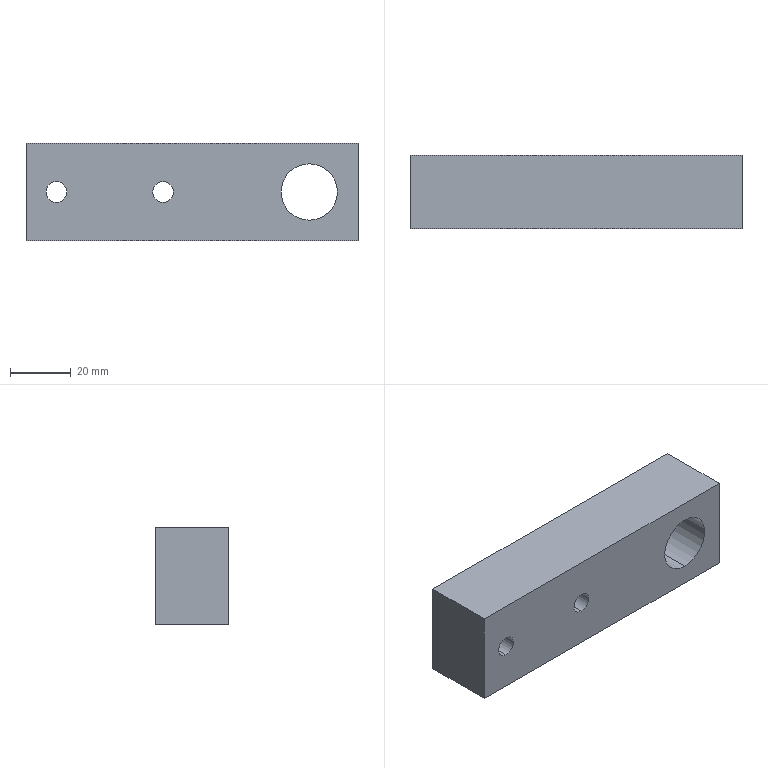Part | STEP file | PN_0035 (buffer fixed block) | 1 solid | 12 faces | box 109 x 24 x 32 mm | volume 75518 mm3 | cylinder 6 | plane 6 | commonest cylinder face diameters 6.8 x4 18.5 x2
STEP:
#1=CARTESIAN_POINT('',(0.,0.,0.));
#2=DIRECTION('',(0.,0.,1.));
#3=DIRECTION('',(1.,0.,0.));
#4=AXIS2_PLACEMENT_3D('',#1,#2,#3);
#5=CARTESIAN_POINT('',(10.,-12.,3.4));
#6=VERTEX_POINT('',#5);
#7=CARTESIAN_POINT('',(10.,12.,3.4));
#8=VERTEX_POINT('',#7);
#9=CARTESIAN_POINT('',(10.,12.,3.4));
#10=DIRECTION('',(0.,1.,0.));
#11=VECTOR('',#10,1.);
#12=LINE('',#9,#11);
#13=CARTESIAN_POINT('',(10.,12.,0.));
#14=DIRECTION('',(0.,1.,0.));
#15=DIRECTION('',(0.,0.,1.));
#16=AXIS2_PLACEMENT_3D('',#13,#14,#15);
#17=CYLINDRICAL_SURFACE('',#16,3.4);
#18=CARTESIAN_POINT('',(6.283,0.));
#19=DIRECTION('',(0.,1.));
#20=VECTOR('',#19,1.);
#21=LINE('',#18,#20);
#22=(GEOMETRIC_REPRESENTATION_CONTEXT(2)PARAMETRIC_REPRESENTATION_CONTEXT()REPRESENTATION_CONTEXT('',''));
#23=DEFINITIONAL_REPRESENTATION('',(#21),#22);
#24=PCURVE('',#17,#23);
#25=CARTESIAN_POINT('',(10.,12.,0.));
#26=DIRECTION('',(0.,1.,0.));
#27=DIRECTION('',(0.,0.,1.));
#28=AXIS2_PLACEMENT_3D('',#25,#26,#27);
#29=CYLINDRICAL_SURFACE('',#28,3.4);
#30=CARTESIAN_POINT('',(0.,0.));
#31=DIRECTION('',(0.,1.));
#32=VECTOR('',#31,1.);
#33=LINE('',#30,#32);
#34=(GEOMETRIC_REPRESENTATION_CONTEXT(2)PARAMETRIC_REPRESENTATION_CONTEXT()REPRESENTATION_CONTEXT('',''));
#35=DEFINITIONAL_REPRESENTATION('',(#33),#34);
#36=PCURVE('',#29,#35);
#37=SURFACE_CURVE('',#12,(#24,#36),.PCURVE_S1.);
#38=EDGE_CURVE('',#6,#8,#37,.T.);
#39=ORIENTED_EDGE('',*,*,#38,.T.);
#40=CARTESIAN_POINT('',(10.,12.,-3.4));
#41=VERTEX_POINT('',#40);
#42=CARTESIAN_POINT('',(10.,12.,0.));
#43=DIRECTION('',(0.,1.,0.));
#44=DIRECTION('',(0.,0.,1.));
#45=AXIS2_PLACEMENT_3D('',#42,#43,#44);
#46=CIRCLE('',#45,3.4);
#47=CARTESIAN_POINT('',(0.,0.));
#48=DIRECTION('',(1.,0.));
#49=VECTOR('',#48,1.);
#50=LINE('',#47,#49);
#51=(GEOMETRIC_REPRESENTATION_CONTEXT(2)PARAMETRIC_REPRESENTATION_CONTEXT()REPRESENTATION_CONTEXT('',''));
#52=DEFINITIONAL_REPRESENTATION('',(#50),#51);
#53=PCURVE('',#17,#52);
#54=CARTESIAN_POINT('',(0.,12.,16.));
#55=DIRECTION('',(0.,-1.,0.));
#56=DIRECTION('',(0.,0.,-1.));
#57=AXIS2_PLACEMENT_3D('',#54,#55,#56);
#58=PLANE('',#57);
#59=CARTESIAN_POINT('',(12.6,10.));
#60=CARTESIAN_POINT('',(12.6,15.889));
#61=CARTESIAN_POINT('',(17.7,12.944));
#62=CARTESIAN_POINT('',(22.8,10.));
#63=CARTESIAN_POINT('',(17.7,7.056));
#64=CARTESIAN_POINT('',(12.6,4.111));
#65=CARTESIAN_POINT('',(12.6,10.));
#66=(BOUNDED_CURVE()B_SPLINE_CURVE(2,(#59,#60,#61,#62,#63,#64,#65),.UNSPECIFIED.,.T.,.F.)B_SPLINE_CURVE_WITH_KNOTS((1,2,2,2,2,1),(-2.094,0.,2.094,4.189,6.283,8.378),.UNSPECIFIED.)CURVE()GEOMETRIC_REPRESENTATION_ITEM()RATIONAL_B_SPLINE_CURVE((1.,0.5,1.,0.5,1.,0.5,1.))REPRESENTATION_ITEM(''));
#67=(GEOMETRIC_REPRESENTATION_CONTEXT(2)PARAMETRIC_REPRESENTATION_CONTEXT()REPRESENTATION_CONTEXT('',''));
#68=DEFINITIONAL_REPRESENTATION('',(#66),#67);
#69=PCURVE('',#58,#68);
#70=SURFACE_CURVE('',#46,(#53,#69),.PCURVE_S1.);
#71=EDGE_CURVE('',#41,#8,#70,.T.);
#72=ORIENTED_EDGE('',*,*,#71,.F.);
#73=CARTESIAN_POINT('',(10.,-12.,-3.4));
#74=VERTEX_POINT('',#73);
#75=CARTESIAN_POINT('',(10.,12.,-3.4));
#76=DIRECTION('',(0.,1.,0.));
#77=VECTOR('',#76,1.);
#78=LINE('',#75,#77);
#79=CARTESIAN_POINT('',(3.142,0.));
#80=DIRECTION('',(0.,1.));
#81=VECTOR('',#80,1.);
#82=LINE('',#79,#81);
#83=(GEOMETRIC_REPRESENTATION_CONTEXT(2)PARAMETRIC_REPRESENTATION_CONTEXT()REPRESENTATION_CONTEXT('',''));
#84=DEFINITIONAL_REPRESENTATION('',(#82),#83);
#85=PCURVE('',#17,#84);
#86=CARTESIAN_POINT('',(3.142,0.));
#87=DIRECTION('',(0.,1.));
#88=VECTOR('',#87,1.);
#89=LINE('',#86,#88);
#90=(GEOMETRIC_REPRESENTATION_CONTEXT(2)PARAMETRIC_REPRESENTATION_CONTEXT()REPRESENTATION_CONTEXT('',''));
#91=DEFINITIONAL_REPRESENTATION('',(#89),#90);
#92=PCURVE('',#29,#91);
#93=SURFACE_CURVE('',#78,(#85,#92),.PCURVE_S1.);
#94=EDGE_CURVE('',#74,#41,#93,.T.);
#95=ORIENTED_EDGE('',*,*,#94,.F.);
#96=CARTESIAN_POINT('',(10.,-12.,0.));
#97=DIRECTION('',(0.,1.,0.));
#98=DIRECTION('',(0.,0.,1.));
#99=AXIS2_PLACEMENT_3D('',#96,#97,#98);
#100=CIRCLE('',#99,3.4);
#101=CARTESIAN_POINT('',(0.,-24.));
#102=DIRECTION('',(1.,0.));
#103=VECTOR('',#102,1.);
#104=LINE('',#101,#103);
#105=(GEOMETRIC_REPRESENTATION_CONTEXT(2)PARAMETRIC_REPRESENTATION_CONTEXT()REPRESENTATION_CONTEXT('',''));
#106=DEFINITIONAL_REPRESENTATION('',(#104),#105);
#107=PCURVE('',#17,#106);
#108=CARTESIAN_POINT('',(0.,-12.,16.));
#109=DIRECTION('',(0.,1.,0.));
#110=DIRECTION('',(0.,0.,1.));
#111=AXIS2_PLACEMENT_3D('',#108,#109,#110);
#112=PLANE('',#111);
#113=CARTESIAN_POINT('',(-16.,10.));
#114=DIRECTION('',(1.,0.));
#115=AXIS2_PLACEMENT_2D('',#113,#114);
#116=CIRCLE('',#115,3.4);
#117=(GEOMETRIC_REPRESENTATION_CONTEXT(2)PARAMETRIC_REPRESENTATION_CONTEXT()REPRESENTATION_CONTEXT('',''));
#118=DEFINITIONAL_REPRESENTATION('',(#116),#117);
#119=PCURVE('',#112,#118);
#120=SURFACE_CURVE('',#100,(#107,#119),.PCURVE_S1.);
#121=EDGE_CURVE('',#74,#6,#120,.T.);
#122=ORIENTED_EDGE('',*,*,#121,.T.);
#123=EDGE_LOOP('',(#39,#72,#95,#122));
#124=FACE_BOUND('',#123,.F.);
#125=ADVANCED_FACE('',(#124),#17,.F.);
#126=CARTESIAN_POINT('',(45.,-12.,3.4));
#127=VERTEX_POINT('',#126);
#128=CARTESIAN_POINT('',(45.,12.,3.4));
#129=VERTEX_POINT('',#128);
#130=CARTESIAN_POINT('',(45.,12.,3.4));
#131=DIRECTION('',(0.,1.,0.));
#132=VECTOR('',#131,1.);
#133=LINE('',#130,#132);
#134=CARTESIAN_POINT('',(45.,12.,0.));
#135=DIRECTION('',(0.,1.,0.));
#136=DIRECTION('',(0.,0.,1.));
#137=AXIS2_PLACEMENT_3D('',#134,#135,#136);
#138=CYLINDRICAL_SURFACE('',#137,3.4);
#139=CARTESIAN_POINT('',(6.283,0.));
#140=DIRECTION('',(0.,1.));
#141=VECTOR('',#140,1.);
#142=LINE('',#139,#141);
#143=(GEOMETRIC_REPRESENTATION_CONTEXT(2)PARAMETRIC_REPRESENTATION_CONTEXT()REPRESENTATION_CONTEXT('',''));
#144=DEFINITIONAL_REPRESENTATION('',(#142),#143);
#145=PCURVE('',#138,#144);
#146=CARTESIAN_POINT('',(45.,12.,0.));
#147=DIRECTION('',(0.,1.,0.));
#148=DIRECTION('',(0.,0.,1.));
#149=AXIS2_PLACEMENT_3D('',#146,#147,#148);
#150=CYLINDRICAL_SURFACE('',#149,3.4);
#151=CARTESIAN_POINT('',(0.,0.));
#152=DIRECTION('',(0.,1.));
#153=VECTOR('',#152,1.);
#154=LINE('',#151,#153);
#155=(GEOMETRIC_REPRESENTATION_CONTEXT(2)PARAMETRIC_REPRESENTATION_CONTEXT()REPRESENTATION_CONTEXT('',''));
#156=DEFINITIONAL_REPRESENTATION('',(#154),#155);
#157=PCURVE('',#150,#156);
#158=SURFACE_CURVE('',#133,(#145,#157),.PCURVE_S1.);
#159=EDGE_CURVE('',#127,#129,#158,.T.);
#160=ORIENTED_EDGE('',*,*,#159,.T.);
#161=CARTESIAN_POINT('',(45.,12.,-3.4));
#162=VERTEX_POINT('',#161);
#163=CARTESIAN_POINT('',(45.,12.,0.));
#164=DIRECTION('',(0.,1.,0.));
#165=DIRECTION('',(0.,0.,1.));
#166=AXIS2_PLACEMENT_3D('',#163,#164,#165);
#167=CIRCLE('',#166,3.4);
#168=CARTESIAN_POINT('',(0.,0.));
#169=DIRECTION('',(1.,0.));
#170=VECTOR('',#169,1.);
#171=LINE('',#168,#170);
#172=(GEOMETRIC_REPRESENTATION_CONTEXT(2)PARAMETRIC_REPRESENTATION_CONTEXT()REPRESENTATION_CONTEXT('',''));
#173=DEFINITIONAL_REPRESENTATION('',(#171),#172);
#174=PCURVE('',#138,#173);
#175=CARTESIAN_POINT('',(12.6,45.));
#176=CARTESIAN_POINT('',(12.6,50.889));
#177=CARTESIAN_POINT('',(17.7,47.944));
#178=CARTESIAN_POINT('',(22.8,45.));
#179=CARTESIAN_POINT('',(17.7,42.056));
#180=CARTESIAN_POINT('',(12.6,39.111));
#181=CARTESIAN_POINT('',(12.6,45.));
#182=(BOUNDED_CURVE()B_SPLINE_CURVE(2,(#175,#176,#177,#178,#179,#180,#181),.UNSPECIFIED.,.T.,.F.)B_SPLINE_CURVE_WITH_KNOTS((1,2,2,2,2,1),(-2.094,0.,2.094,4.189,6.283,8.378),.UNSPECIFIED.)CURVE()GEOMETRIC_REPRESENTATION_ITEM()RATIONAL_B_SPLINE_CURVE((1.,0.5,1.,0.5,1.,0.5,1.))REPRESENTATION_ITEM(''));
#183=(GEOMETRIC_REPRESENTATION_CONTEXT(2)PARAMETRIC_REPRESENTATION_CONTEXT()REPRESENTATION_CONTEXT('',''));
#184=DEFINITIONAL_REPRESENTATION('',(#182),#183);
#185=PCURVE('',#58,#184);
#186=SURFACE_CURVE('',#167,(#174,#185),.PCURVE_S1.);
#187=EDGE_CURVE('',#162,#129,#186,.T.);
#188=ORIENTED_EDGE('',*,*,#187,.F.);
#189=CARTESIAN_POINT('',(45.,-12.,-3.4));
#190=VERTEX_POINT('',#189);
#191=CARTESIAN_POINT('',(45.,12.,-3.4));
#192=DIRECTION('',(0.,1.,0.));
#193=VECTOR('',#192,1.);
#194=LINE('',#191,#193);
#195=CARTESIAN_POINT('',(3.142,0.));
#196=DIRECTION('',(0.,1.));
#197=VECTOR('',#196,1.);
#198=LINE('',#195,#197);
#199=(GEOMETRIC_REPRESENTATION_CONTEXT(2)PARAMETRIC_REPRESENTATION_CONTEXT()REPRESENTATION_CONTEXT('',''));
#200=DEFINITIONAL_REPRESENTATION('',(#198),#199);
#201=PCURVE('',#138,#200);
#202=CARTESIAN_POINT('',(3.142,0.));
#203=DIRECTION('',(0.,1.));
#204=VECTOR('',#203,1.);
#205=LINE('',#202,#204);
#206=(GEOMETRIC_REPRESENTATION_CONTEXT(2)PARAMETRIC_REPRESENTATION_CONTEXT()REPRESENTATION_CONTEXT('',''));
#207=DEFINITIONAL_REPRESENTATION('',(#205),#206);
#208=PCURVE('',#150,#207);
#209=SURFACE_CURVE('',#194,(#201,#208),.PCURVE_S1.);
#210=EDGE_CURVE('',#190,#162,#209,.T.);
#211=ORIENTED_EDGE('',*,*,#210,.F.);
#212=CARTESIAN_POINT('',(45.,-12.,0.));
#213=DIRECTION('',(0.,1.,0.));
#214=DIRECTION('',(0.,0.,1.));
#215=AXIS2_PLACEMENT_3D('',#212,#213,#214);
#216=CIRCLE('',#215,3.4);
#217=CARTESIAN_POINT('',(0.,-24.));
#218=DIRECTION('',(1.,0.));
#219=VECTOR('',#218,1.);
#220=LINE('',#217,#219);
#221=(GEOMETRIC_REPRESENTATION_CONTEXT(2)PARAMETRIC_REPRESENTATION_CONTEXT()REPRESENTATION_CONTEXT('',''));
#222=DEFINITIONAL_REPRESENTATION('',(#220),#221);
#223=PCURVE('',#138,#222);
#224=CARTESIAN_POINT('',(-16.,45.));
#225=DIRECTION('',(1.,0.));
#226=AXIS2_PLACEMENT_2D('',#224,#225);
#227=CIRCLE('',#226,3.4);
#228=(GEOMETRIC_REPRESENTATION_CONTEXT(2)PARAMETRIC_REPRESENTATION_CONTEXT()REPRESENTATION_CONTEXT('',''));
#229=DEFINITIONAL_REPRESENTATION('',(#227),#228);
#230=PCURVE('',#112,#229);
#231=SURFACE_CURVE('',#216,(#223,#230),.PCURVE_S1.);
#232=EDGE_CURVE('',#190,#127,#231,.T.);
#233=ORIENTED_EDGE('',*,*,#232,.T.);
#234=EDGE_LOOP('',(#160,#188,#211,#233));
#235=FACE_BOUND('',#234,.F.);
#236=ADVANCED_FACE('',(#235),#138,.F.);
#237=CARTESIAN_POINT('',(93.,-12.,9.25));
#238=VERTEX_POINT('',#237);
#239=CARTESIAN_POINT('',(93.,12.,9.25));
#240=VERTEX_POINT('',#239);
#241=CARTESIAN_POINT('',(93.,12.,9.25));
#242=DIRECTION('',(0.,1.,0.));
#243=VECTOR('',#242,1.);
#244=LINE('',#241,#243);
#245=CARTESIAN_POINT('',(93.,12.,0.));
#246=DIRECTION('',(0.,1.,0.));
#247=DIRECTION('',(0.,0.,1.));
#248=AXIS2_PLACEMENT_3D('',#245,#246,#247);
#249=CYLINDRICAL_SURFACE('',#248,9.25);
#250=CARTESIAN_POINT('',(6.283,0.));
#251=DIRECTION('',(0.,1.));
#252=VECTOR('',#251,1.);
#253=LINE('',#250,#252);
#254=(GEOMETRIC_REPRESENTATION_CONTEXT(2)PARAMETRIC_REPRESENTATION_CONTEXT()REPRESENTATION_CONTEXT('',''));
#255=DEFINITIONAL_REPRESENTATION('',(#253),#254);
#256=PCURVE('',#249,#255);
#257=CARTESIAN_POINT('',(93.,12.,0.));
#258=DIRECTION('',(0.,1.,0.));
#259=DIRECTION('',(0.,0.,1.));
#260=AXIS2_PLACEMENT_3D('',#257,#258,#259);
#261=CYLINDRICAL_SURFACE('',#260,9.25);
#262=CARTESIAN_POINT('',(0.,0.));
#263=DIRECTION('',(0.,1.));
#264=VECTOR('',#263,1.);
#265=LINE('',#262,#264);
#266=(GEOMETRIC_REPRESENTATION_CONTEXT(2)PARAMETRIC_REPRESENTATION_CONTEXT()REPRESENTATION_CONTEXT('',''));
#267=DEFINITIONAL_REPRESENTATION('',(#265),#266);
#268=PCURVE('',#261,#267);
#269=SURFACE_CURVE('',#244,(#256,#268),.PCURVE_S1.);
#270=EDGE_CURVE('',#238,#240,#269,.T.);
#271=ORIENTED_EDGE('',*,*,#270,.T.);
#272=CARTESIAN_POINT('',(93.,12.,-9.25));
#273=VERTEX_POINT('',#272);
#274=CARTESIAN_POINT('',(93.,12.,0.));
#275=DIRECTION('',(0.,1.,0.));
#276=DIRECTION('',(0.,0.,1.));
#277=AXIS2_PLACEMENT_3D('',#274,#275,#276);
#278=CIRCLE('',#277,9.25);
#279=CARTESIAN_POINT('',(0.,0.));
#280=DIRECTION('',(1.,0.));
#281=VECTOR('',#280,1.);
#282=LINE('',#279,#281);
#283=(GEOMETRIC_REPRESENTATION_CONTEXT(2)PARAMETRIC_REPRESENTATION_CONTEXT()REPRESENTATION_CONTEXT('',''));
#284=DEFINITIONAL_REPRESENTATION('',(#282),#283);
#285=PCURVE('',#249,#284);
#286=CARTESIAN_POINT('',(6.75,93.));
#287=CARTESIAN_POINT('',(6.75,109.021));
#288=CARTESIAN_POINT('',(20.625,101.011));
#289=CARTESIAN_POINT('',(34.5,93.));
#290=CARTESIAN_POINT('',(20.625,84.989));
#291=CARTESIAN_POINT('',(6.75,76.979));
#292=CARTESIAN_POINT('',(6.75,93.));
#293=(BOUNDED_CURVE()B_SPLINE_CURVE(2,(#286,#287,#288,#289,#290,#291,#292),.UNSPECIFIED.,.T.,.F.)B_SPLINE_CURVE_WITH_KNOTS((1,2,2,2,2,1),(-2.094,0.,2.094,4.189,6.283,8.378),.UNSPECIFIED.)CURVE()GEOMETRIC_REPRESENTATION_ITEM()RATIONAL_B_SPLINE_CURVE((1.,0.5,1.,0.5,1.,0.5,1.))REPRESENTATION_ITEM(''));
#294=(GEOMETRIC_REPRESENTATION_CONTEXT(2)PARAMETRIC_REPRESENTATION_CONTEXT()REPRESENTATION_CONTEXT('',''));
#295=DEFINITIONAL_REPRESENTATION('',(#293),#294);
#296=PCURVE('',#58,#295);
#297=SURFACE_CURVE('',#278,(#285,#296),.PCURVE_S1.);
#298=EDGE_CURVE('',#273,#240,#297,.T.);
#299=ORIENTED_EDGE('',*,*,#298,.F.);
#300=CARTESIAN_POINT('',(93.,-12.,-9.25));
#301=VERTEX_POINT('',#300);
#302=CARTESIAN_POINT('',(93.,12.,-9.25));
#303=DIRECTION('',(0.,1.,0.));
#304=VECTOR('',#303,1.);
#305=LINE('',#302,#304);
#306=CARTESIAN_POINT('',(3.142,0.));
#307=DIRECTION('',(0.,1.));
#308=VECTOR('',#307,1.);
#309=LINE('',#306,#308);
#310=(GEOMETRIC_REPRESENTATION_CONTEXT(2)PARAMETRIC_REPRESENTATION_CONTEXT()REPRESENTATION_CONTEXT('',''));
#311=DEFINITIONAL_REPRESENTATION('',(#309),#310);
#312=PCURVE('',#249,#311);
#313=CARTESIAN_POINT('',(3.142,0.));
#314=DIRECTION('',(0.,1.));
#315=VECTOR('',#314,1.);
#316=LINE('',#313,#315);
#317=(GEOMETRIC_REPRESENTATION_CONTEXT(2)PARAMETRIC_REPRESENTATION_CONTEXT()REPRESENTATION_CONTEXT('',''));
#318=DEFINITIONAL_REPRESENTATION('',(#316),#317);
#319=PCURVE('',#261,#318);
#320=SURFACE_CURVE('',#305,(#312,#319),.PCURVE_S1.);
#321=EDGE_CURVE('',#301,#273,#320,.T.);
#322=ORIENTED_EDGE('',*,*,#321,.F.);
#323=CARTESIAN_POINT('',(93.,-12.,0.));
#324=DIRECTION('',(0.,1.,0.));
#325=DIRECTION('',(0.,0.,1.));
#326=AXIS2_PLACEMENT_3D('',#323,#324,#325);
#327=CIRCLE('',#326,9.25);
#328=CARTESIAN_POINT('',(0.,-24.));
#329=DIRECTION('',(1.,0.));
#330=VECTOR('',#329,1.);
#331=LINE('',#328,#330);
#332=(GEOMETRIC_REPRESENTATION_CONTEXT(2)PARAMETRIC_REPRESENTATION_CONTEXT()REPRESENTATION_CONTEXT('',''));
#333=DEFINITIONAL_REPRESENTATION('',(#331),#332);
#334=PCURVE('',#249,#333);
#335=CARTESIAN_POINT('',(-16.,93.));
#336=DIRECTION('',(1.,0.));
#337=AXIS2_PLACEMENT_2D('',#335,#336);
#338=CIRCLE('',#337,9.25);
#339=(GEOMETRIC_REPRESENTATION_CONTEXT(2)PARAMETRIC_REPRESENTATION_CONTEXT()REPRESENTATION_CONTEXT('',''));
#340=DEFINITIONAL_REPRESENTATION('',(#338),#339);
#341=PCURVE('',#112,#340);
#342=SURFACE_CURVE('',#327,(#334,#341),.PCURVE_S1.);
#343=EDGE_CURVE('',#301,#238,#342,.T.);
#344=ORIENTED_EDGE('',*,*,#343,.T.);
#345=EDGE_LOOP('',(#271,#299,#322,#344));
#346=FACE_BOUND('',#345,.F.);
#347=ADVANCED_FACE('',(#346),#249,.F.);
#348=CARTESIAN_POINT('',(0.,12.,-16.));
#349=VERTEX_POINT('',#348);
#350=CARTESIAN_POINT('',(0.,-12.,-16.));
#351=VERTEX_POINT('',#350);
#352=CARTESIAN_POINT('',(0.,-12.,-16.));
#353=DIRECTION('',(0.,-1.,0.));
#354=VECTOR('',#353,1.);
#355=LINE('',#352,#354);
#356=CARTESIAN_POINT('',(0.,-12.,16.));
#357=DIRECTION('',(1.,0.,0.));
#358=DIRECTION('',(0.,0.,-1.));
#359=AXIS2_PLACEMENT_3D('',#356,#357,#358);
#360=PLANE('',#359);
#361=CARTESIAN_POINT('',(32.,0.));
#362=DIRECTION('',(0.,-1.));
#363=VECTOR('',#362,1.);
#364=LINE('',#361,#363);
#365=(GEOMETRIC_REPRESENTATION_CONTEXT(2)PARAMETRIC_REPRESENTATION_CONTEXT()REPRESENTATION_CONTEXT('',''));
#366=DEFINITIONAL_REPRESENTATION('',(#364),#365);
#367=PCURVE('',#360,#366);
#368=CARTESIAN_POINT('',(0.,0.,-16.));
#369=DIRECTION('',(0.,0.,-1.));
#370=DIRECTION('',(-1.,0.,0.));
#371=AXIS2_PLACEMENT_3D('',#368,#369,#370);
#372=PLANE('',#371);
#373=CARTESIAN_POINT('',(0.,-12.));
#374=DIRECTION('',(0.,-1.));
#375=VECTOR('',#374,1.);
#376=LINE('',#373,#375);
#377=(GEOMETRIC_REPRESENTATION_CONTEXT(2)PARAMETRIC_REPRESENTATION_CONTEXT()REPRESENTATION_CONTEXT('',''));
#378=DEFINITIONAL_REPRESENTATION('',(#376),#377);
#379=PCURVE('',#372,#378);
#380=SURFACE_CURVE('',#355,(#367,#379),.PCURVE_S1.);
#381=EDGE_CURVE('',#349,#351,#380,.T.);
#382=ORIENTED_EDGE('',*,*,#381,.T.);
#383=CARTESIAN_POINT('',(0.,-12.,16.));
#384=VERTEX_POINT('',#383);
#385=CARTESIAN_POINT('',(0.,-12.,16.));
#386=DIRECTION('',(0.,0.,-1.));
#387=VECTOR('',#386,1.);
#388=LINE('',#385,#387);
#389=CARTESIAN_POINT('',(0.,0.));
#390=DIRECTION('',(1.,0.));
#391=VECTOR('',#390,1.);
#392=LINE('',#389,#391);
#393=(GEOMETRIC_REPRESENTATION_CONTEXT(2)PARAMETRIC_REPRESENTATION_CONTEXT()REPRESENTATION_CONTEXT('',''));
#394=DEFINITIONAL_REPRESENTATION('',(#392),#393);
#395=PCURVE('',#360,#394);
#396=CARTESIAN_POINT('',(0.,0.));
#397=DIRECTION('',(-1.,0.));
#398=VECTOR('',#397,1.);
#399=LINE('',#396,#398);
#400=(GEOMETRIC_REPRESENTATION_CONTEXT(2)PARAMETRIC_REPRESENTATION_CONTEXT()REPRESENTATION_CONTEXT('',''));
#401=DEFINITIONAL_REPRESENTATION('',(#399),#400);
#402=PCURVE('',#112,#401);
#403=SURFACE_CURVE('',#388,(#395,#402),.PCURVE_S1.);
#404=EDGE_CURVE('',#384,#351,#403,.T.);
#405=ORIENTED_EDGE('',*,*,#404,.F.);
#406=CARTESIAN_POINT('',(0.,12.,16.));
#407=VERTEX_POINT('',#406);
#408=CARTESIAN_POINT('',(0.,-12.,16.));
#409=DIRECTION('',(0.,-1.,0.));
#410=VECTOR('',#409,1.);
#411=LINE('',#408,#410);
#412=CARTESIAN_POINT('',(0.,0.));
#413=DIRECTION('',(0.,-1.));
#414=VECTOR('',#413,1.);
#415=LINE('',#412,#414);
#416=(GEOMETRIC_REPRESENTATION_CONTEXT(2)PARAMETRIC_REPRESENTATION_CONTEXT()REPRESENTATION_CONTEXT('',''));
#417=DEFINITIONAL_REPRESENTATION('',(#415),#416);
#418=PCURVE('',#360,#417);
#419=CARTESIAN_POINT('',(0.,0.,16.));
#420=DIRECTION('',(0.,0.,-1.));
#421=DIRECTION('',(-1.,0.,0.));
#422=AXIS2_PLACEMENT_3D('',#419,#420,#421);
#423=PLANE('',#422);
#424=CARTESIAN_POINT('',(0.,-12.));
#425=DIRECTION('',(0.,-1.));
#426=VECTOR('',#425,1.);
#427=LINE('',#424,#426);
#428=(GEOMETRIC_REPRESENTATION_CONTEXT(2)PARAMETRIC_REPRESENTATION_CONTEXT()REPRESENTATION_CONTEXT('',''));
#429=DEFINITIONAL_REPRESENTATION('',(#427),#428);
#430=PCURVE('',#423,#429);
#431=SURFACE_CURVE('',#411,(#418,#430),.PCURVE_S1.);
#432=EDGE_CURVE('',#407,#384,#431,.T.);
#433=ORIENTED_EDGE('',*,*,#432,.F.);
#434=CARTESIAN_POINT('',(0.,12.,16.));
#435=DIRECTION('',(0.,0.,-1.));
#436=VECTOR('',#435,1.);
#437=LINE('',#434,#436);
#438=CARTESIAN_POINT('',(0.,24.));
#439=DIRECTION('',(1.,0.));
#440=VECTOR('',#439,1.);
#441=LINE('',#438,#440);
#442=(GEOMETRIC_REPRESENTATION_CONTEXT(2)PARAMETRIC_REPRESENTATION_CONTEXT()REPRESENTATION_CONTEXT('',''));
#443=DEFINITIONAL_REPRESENTATION('',(#441),#442);
#444=PCURVE('',#360,#443);
#445=CARTESIAN_POINT('',(0.,0.));
#446=DIRECTION('',(1.,0.));
#447=VECTOR('',#446,1.);
#448=LINE('',#445,#447);
#449=(GEOMETRIC_REPRESENTATION_CONTEXT(2)PARAMETRIC_REPRESENTATION_CONTEXT()REPRESENTATION_CONTEXT('',''));
#450=DEFINITIONAL_REPRESENTATION('',(#448),#449);
#451=PCURVE('',#58,#450);
#452=SURFACE_CURVE('',#437,(#444,#451),.PCURVE_S1.);
#453=EDGE_CURVE('',#407,#349,#452,.T.);
#454=ORIENTED_EDGE('',*,*,#453,.T.);
#455=EDGE_LOOP('',(#382,#405,#433,#454));
#456=FACE_BOUND('',#455,.T.);
#457=ADVANCED_FACE('',(#456),#360,.F.);
#458=CARTESIAN_POINT('',(10.,-12.,0.));
#459=DIRECTION('',(0.,1.,0.));
#460=DIRECTION('',(0.,0.,1.));
#461=AXIS2_PLACEMENT_3D('',#458,#459,#460);
#462=CIRCLE('',#461,3.4);
#463=CARTESIAN_POINT('',(-16.,10.));
#464=DIRECTION('',(1.,0.));
#465=AXIS2_PLACEMENT_2D('',#463,#464);
#466=CIRCLE('',#465,3.4);
#467=(GEOMETRIC_REPRESENTATION_CONTEXT(2)PARAMETRIC_REPRESENTATION_CONTEXT()REPRESENTATION_CONTEXT('',''));
#468=DEFINITIONAL_REPRESENTATION('',(#466),#467);
#469=PCURVE('',#112,#468);
#470=CARTESIAN_POINT('',(0.,-24.));
#471=DIRECTION('',(1.,0.));
#472=VECTOR('',#471,1.);
#473=LINE('',#470,#472);
#474=(GEOMETRIC_REPRESENTATION_CONTEXT(2)PARAMETRIC_REPRESENTATION_CONTEXT()REPRESENTATION_CONTEXT('',''));
#475=DEFINITIONAL_REPRESENTATION('',(#473),#474);
#476=PCURVE('',#29,#475);
#477=SURFACE_CURVE('',#462,(#469,#476),.PCURVE_S1.);
#478=EDGE_CURVE('',#6,#74,#477,.T.);
#479=ORIENTED_EDGE('',*,*,#478,.T.);
#480=ORIENTED_EDGE('',*,*,#121,.T.);
#481=EDGE_LOOP('',(#479,#480));
#482=FACE_BOUND('',#481,.T.);
#483=CARTESIAN_POINT('',(45.,-12.,0.));
#484=DIRECTION('',(0.,1.,0.));
#485=DIRECTION('',(0.,0.,1.));
#486=AXIS2_PLACEMENT_3D('',#483,#484,#485);
#487=CIRCLE('',#486,3.4);
#488=CARTESIAN_POINT('',(-16.,45.));
#489=DIRECTION('',(1.,0.));
#490=AXIS2_PLACEMENT_2D('',#488,#489);
#491=CIRCLE('',#490,3.4);
#492=(GEOMETRIC_REPRESENTATION_CONTEXT(2)PARAMETRIC_REPRESENTATION_CONTEXT()REPRESENTATION_CONTEXT('',''));
#493=DEFINITIONAL_REPRESENTATION('',(#491),#492);
#494=PCURVE('',#112,#493);
#495=CARTESIAN_POINT('',(0.,-24.));
#496=DIRECTION('',(1.,0.));
#497=VECTOR('',#496,1.);
#498=LINE('',#495,#497);
#499=(GEOMETRIC_REPRESENTATION_CONTEXT(2)PARAMETRIC_REPRESENTATION_CONTEXT()REPRESENTATION_CONTEXT('',''));
#500=DEFINITIONAL_REPRESENTATION('',(#498),#499);
#501=PCURVE('',#150,#500);
#502=SURFACE_CURVE('',#487,(#494,#501),.PCURVE_S1.);
#503=EDGE_CURVE('',#127,#190,#502,.T.);
#504=ORIENTED_EDGE('',*,*,#503,.T.);
#505=ORIENTED_EDGE('',*,*,#232,.T.);
#506=EDGE_LOOP('',(#504,#505));
#507=FACE_BOUND('',#506,.T.);
#508=CARTESIAN_POINT('',(93.,-12.,0.));
#509=DIRECTION('',(0.,1.,0.));
#510=DIRECTION('',(0.,0.,1.));
#511=AXIS2_PLACEMENT_3D('',#508,#509,#510);
#512=CIRCLE('',#511,9.25);
#513=CARTESIAN_POINT('',(-16.,93.));
#514=DIRECTION('',(1.,0.));
#515=AXIS2_PLACEMENT_2D('',#513,#514);
#516=CIRCLE('',#515,9.25);
#517=(GEOMETRIC_REPRESENTATION_CONTEXT(2)PARAMETRIC_REPRESENTATION_CONTEXT()REPRESENTATION_CONTEXT('',''));
#518=DEFINITIONAL_REPRESENTATION('',(#516),#517);
#519=PCURVE('',#112,#518);
#520=CARTESIAN_POINT('',(0.,-24.));
#521=DIRECTION('',(1.,0.));
#522=VECTOR('',#521,1.);
#523=LINE('',#520,#522);
#524=(GEOMETRIC_REPRESENTATION_CONTEXT(2)PARAMETRIC_REPRESENTATION_CONTEXT()REPRESENTATION_CONTEXT('',''));
#525=DEFINITIONAL_REPRESENTATION('',(#523),#524);
#526=PCURVE('',#261,#525);
#527=SURFACE_CURVE('',#512,(#519,#526),.PCURVE_S1.);
#528=EDGE_CURVE('',#238,#301,#527,.T.);
#529=ORIENTED_EDGE('',*,*,#528,.T.);
#530=ORIENTED_EDGE('',*,*,#343,.T.);
#531=EDGE_LOOP('',(#529,#530));
#532=FACE_BOUND('',#531,.T.);
#533=CARTESIAN_POINT('',(109.,-12.,-16.));
#534=VERTEX_POINT('',#533);
#535=CARTESIAN_POINT('',(0.,-12.,-16.));
#536=DIRECTION('',(1.,0.,0.));
#537=VECTOR('',#536,1.);
#538=LINE('',#535,#537);
#539=CARTESIAN_POINT('',(-32.,0.));
#540=DIRECTION('',(0.,1.));
#541=VECTOR('',#540,1.);
#542=LINE('',#539,#541);
#543=(GEOMETRIC_REPRESENTATION_CONTEXT(2)PARAMETRIC_REPRESENTATION_CONTEXT()REPRESENTATION_CONTEXT('',''));
#544=DEFINITIONAL_REPRESENTATION('',(#542),#543);
#545=PCURVE('',#112,#544);
#546=CARTESIAN_POINT('',(0.,-12.));
#547=DIRECTION('',(-1.,0.));
#548=VECTOR('',#547,1.);
#549=LINE('',#546,#548);
#550=(GEOMETRIC_REPRESENTATION_CONTEXT(2)PARAMETRIC_REPRESENTATION_CONTEXT()REPRESENTATION_CONTEXT('',''));
#551=DEFINITIONAL_REPRESENTATION('',(#549),#550);
#552=PCURVE('',#372,#551);
#553=SURFACE_CURVE('',#538,(#545,#552),.PCURVE_S1.);
#554=EDGE_CURVE('',#351,#534,#553,.T.);
#555=ORIENTED_EDGE('',*,*,#554,.T.);
#556=CARTESIAN_POINT('',(109.,-12.,16.));
#557=VERTEX_POINT('',#556);
#558=CARTESIAN_POINT('',(109.,-12.,16.));
#559=DIRECTION('',(0.,0.,-1.));
#560=VECTOR('',#559,1.);
#561=LINE('',#558,#560);
#562=CARTESIAN_POINT('',(0.,109.));
#563=DIRECTION('',(-1.,0.));
#564=VECTOR('',#563,1.);
#565=LINE('',#562,#564);
#566=(GEOMETRIC_REPRESENTATION_CONTEXT(2)PARAMETRIC_REPRESENTATION_CONTEXT()REPRESENTATION_CONTEXT('',''));
#567=DEFINITIONAL_REPRESENTATION('',(#565),#566);
#568=PCURVE('',#112,#567);
#569=CARTESIAN_POINT('',(109.,-12.,16.));
#570=DIRECTION('',(-1.,0.,0.));
#571=DIRECTION('',(0.,0.,1.));
#572=AXIS2_PLACEMENT_3D('',#569,#570,#571);
#573=PLANE('',#572);
#574=CARTESIAN_POINT('',(0.,0.));
#575=DIRECTION('',(-1.,0.));
#576=VECTOR('',#575,1.);
#577=LINE('',#574,#576);
#578=(GEOMETRIC_REPRESENTATION_CONTEXT(2)PARAMETRIC_REPRESENTATION_CONTEXT()REPRESENTATION_CONTEXT('',''));
#579=DEFINITIONAL_REPRESENTATION('',(#577),#578);
#580=PCURVE('',#573,#579);
#581=SURFACE_CURVE('',#561,(#568,#580),.PCURVE_S1.);
#582=EDGE_CURVE('',#557,#534,#581,.T.);
#583=ORIENTED_EDGE('',*,*,#582,.F.);
#584=CARTESIAN_POINT('',(0.,-12.,16.));
#585=DIRECTION('',(1.,0.,0.));
#586=VECTOR('',#585,1.);
#587=LINE('',#584,#586);
#588=CARTESIAN_POINT('',(0.,0.));
#589=DIRECTION('',(0.,1.));
#590=VECTOR('',#589,1.);
#591=LINE('',#588,#590);
#592=(GEOMETRIC_REPRESENTATION_CONTEXT(2)PARAMETRIC_REPRESENTATION_CONTEXT()REPRESENTATION_CONTEXT('',''));
#593=DEFINITIONAL_REPRESENTATION('',(#591),#592);
#594=PCURVE('',#112,#593);
#595=CARTESIAN_POINT('',(0.,-12.));
#596=DIRECTION('',(-1.,0.));
#597=VECTOR('',#596,1.);
#598=LINE('',#595,#597);
#599=(GEOMETRIC_REPRESENTATION_CONTEXT(2)PARAMETRIC_REPRESENTATION_CONTEXT()REPRESENTATION_CONTEXT('',''));
#600=DEFINITIONAL_REPRESENTATION('',(#598),#599);
#601=PCURVE('',#423,#600);
#602=SURFACE_CURVE('',#587,(#594,#601),.PCURVE_S1.);
#603=EDGE_CURVE('',#384,#557,#602,.T.);
#604=ORIENTED_EDGE('',*,*,#603,.F.);
#605=ORIENTED_EDGE('',*,*,#404,.T.);
#606=EDGE_LOOP('',(#555,#583,#604,#605));
#607=FACE_BOUND('',#606,.T.);
#608=ADVANCED_FACE('',(#482,#507,#532,#607),#112,.F.);
#609=CARTESIAN_POINT('',(109.,12.,-16.));
#610=VERTEX_POINT('',#609);
#611=CARTESIAN_POINT('',(109.,-12.,-16.));
#612=DIRECTION('',(0.,1.,0.));
#613=VECTOR('',#612,1.);
#614=LINE('',#611,#613);
#615=CARTESIAN_POINT('',(-32.,0.));
#616=DIRECTION('',(0.,1.));
#617=VECTOR('',#616,1.);
#618=LINE('',#615,#617);
#619=(GEOMETRIC_REPRESENTATION_CONTEXT(2)PARAMETRIC_REPRESENTATION_CONTEXT()REPRESENTATION_CONTEXT('',''));
#620=DEFINITIONAL_REPRESENTATION('',(#618),#619);
#621=PCURVE('',#573,#620);
#622=CARTESIAN_POINT('',(-109.,-12.));
#623=DIRECTION('',(0.,1.));
#624=VECTOR('',#623,1.);
#625=LINE('',#622,#624);
#626=(GEOMETRIC_REPRESENTATION_CONTEXT(2)PARAMETRIC_REPRESENTATION_CONTEXT()REPRESENTATION_CONTEXT('',''));
#627=DEFINITIONAL_REPRESENTATION('',(#625),#626);
#628=PCURVE('',#372,#627);
#629=SURFACE_CURVE('',#614,(#621,#628),.PCURVE_S1.);
#630=EDGE_CURVE('',#534,#610,#629,.T.);
#631=ORIENTED_EDGE('',*,*,#630,.T.);
#632=CARTESIAN_POINT('',(109.,12.,16.));
#633=VERTEX_POINT('',#632);
#634=CARTESIAN_POINT('',(109.,12.,16.));
#635=DIRECTION('',(0.,0.,-1.));
#636=VECTOR('',#635,1.);
#637=LINE('',#634,#636);
#638=CARTESIAN_POINT('',(0.,24.));
#639=DIRECTION('',(-1.,0.));
#640=VECTOR('',#639,1.);
#641=LINE('',#638,#640);
#642=(GEOMETRIC_REPRESENTATION_CONTEXT(2)PARAMETRIC_REPRESENTATION_CONTEXT()REPRESENTATION_CONTEXT('',''));
#643=DEFINITIONAL_REPRESENTATION('',(#641),#642);
#644=PCURVE('',#573,#643);
#645=CARTESIAN_POINT('',(0.,109.));
#646=DIRECTION('',(1.,0.));
#647=VECTOR('',#646,1.);
#648=LINE('',#645,#647);
#649=(GEOMETRIC_REPRESENTATION_CONTEXT(2)PARAMETRIC_REPRESENTATION_CONTEXT()REPRESENTATION_CONTEXT('',''));
#650=DEFINITIONAL_REPRESENTATION('',(#648),#649);
#651=PCURVE('',#58,#650);
#652=SURFACE_CURVE('',#637,(#644,#651),.PCURVE_S1.);
#653=EDGE_CURVE('',#633,#610,#652,.T.);
#654=ORIENTED_EDGE('',*,*,#653,.F.);
#655=CARTESIAN_POINT('',(109.,-12.,16.));
#656=DIRECTION('',(0.,1.,0.));
#657=VECTOR('',#656,1.);
#658=LINE('',#655,#657);
#659=CARTESIAN_POINT('',(0.,0.));
#660=DIRECTION('',(0.,1.));
#661=VECTOR('',#660,1.);
#662=LINE('',#659,#661);
#663=(GEOMETRIC_REPRESENTATION_CONTEXT(2)PARAMETRIC_REPRESENTATION_CONTEXT()REPRESENTATION_CONTEXT('',''));
#664=DEFINITIONAL_REPRESENTATION('',(#662),#663);
#665=PCURVE('',#573,#664);
#666=CARTESIAN_POINT('',(-109.,-12.));
#667=DIRECTION('',(0.,1.));
#668=VECTOR('',#667,1.);
#669=LINE('',#666,#668);
#670=(GEOMETRIC_REPRESENTATION_CONTEXT(2)PARAMETRIC_REPRESENTATION_CONTEXT()REPRESENTATION_CONTEXT('',''));
#671=DEFINITIONAL_REPRESENTATION('',(#669),#670);
#672=PCURVE('',#423,#671);
#673=SURFACE_CURVE('',#658,(#665,#672),.PCURVE_S1.);
#674=EDGE_CURVE('',#557,#633,#673,.T.);
#675=ORIENTED_EDGE('',*,*,#674,.F.);
#676=ORIENTED_EDGE('',*,*,#582,.T.);
#677=EDGE_LOOP('',(#631,#654,#675,#676));
#678=FACE_BOUND('',#677,.T.);
#679=ADVANCED_FACE('',(#678),#573,.F.);
#680=CARTESIAN_POINT('',(10.,12.,0.));
#681=DIRECTION('',(0.,1.,0.));
#682=DIRECTION('',(0.,0.,1.));
#683=AXIS2_PLACEMENT_3D('',#680,#681,#682);
#684=CIRCLE('',#683,3.4);
#685=CARTESIAN_POINT('',(12.6,10.));
#686=CARTESIAN_POINT('',(12.6,15.889));
#687=CARTESIAN_POINT('',(17.7,12.944));
#688=CARTESIAN_POINT('',(22.8,10.));
#689=CARTESIAN_POINT('',(17.7,7.056));
#690=CARTESIAN_POINT('',(12.6,4.111));
#691=CARTESIAN_POINT('',(12.6,10.));
#692=(BOUNDED_CURVE()B_SPLINE_CURVE(2,(#685,#686,#687,#688,#689,#690,#691),.UNSPECIFIED.,.T.,.F.)B_SPLINE_CURVE_WITH_KNOTS((1,2,2,2,2,1),(-2.094,0.,2.094,4.189,6.283,8.378),.UNSPECIFIED.)CURVE()GEOMETRIC_REPRESENTATION_ITEM()RATIONAL_B_SPLINE_CURVE((1.,0.5,1.,0.5,1.,0.5,1.))REPRESENTATION_ITEM(''));
#693=(GEOMETRIC_REPRESENTATION_CONTEXT(2)PARAMETRIC_REPRESENTATION_CONTEXT()REPRESENTATION_CONTEXT('',''));
#694=DEFINITIONAL_REPRESENTATION('',(#692),#693);
#695=PCURVE('',#58,#694);
#696=CARTESIAN_POINT('',(0.,0.));
#697=DIRECTION('',(1.,0.));
#698=VECTOR('',#697,1.);
#699=LINE('',#696,#698);
#700=(GEOMETRIC_REPRESENTATION_CONTEXT(2)PARAMETRIC_REPRESENTATION_CONTEXT()REPRESENTATION_CONTEXT('',''));
#701=DEFINITIONAL_REPRESENTATION('',(#699),#700);
#702=PCURVE('',#29,#701);
#703=SURFACE_CURVE('',#684,(#695,#702),.PCURVE_S1.);
#704=EDGE_CURVE('',#8,#41,#703,.T.);
#705=ORIENTED_EDGE('',*,*,#704,.F.);
#706=ORIENTED_EDGE('',*,*,#71,.F.);
#707=EDGE_LOOP('',(#705,#706));
#708=FACE_BOUND('',#707,.T.);
#709=CARTESIAN_POINT('',(45.,12.,0.));
#710=DIRECTION('',(0.,1.,0.));
#711=DIRECTION('',(0.,0.,1.));
#712=AXIS2_PLACEMENT_3D('',#709,#710,#711);
#713=CIRCLE('',#712,3.4);
#714=CARTESIAN_POINT('',(12.6,45.));
#715=CARTESIAN_POINT('',(12.6,50.889));
#716=CARTESIAN_POINT('',(17.7,47.944));
#717=CARTESIAN_POINT('',(22.8,45.));
#718=CARTESIAN_POINT('',(17.7,42.056));
#719=CARTESIAN_POINT('',(12.6,39.111));
#720=CARTESIAN_POINT('',(12.6,45.));
#721=(BOUNDED_CURVE()B_SPLINE_CURVE(2,(#714,#715,#716,#717,#718,#719,#720),.UNSPECIFIED.,.T.,.F.)B_SPLINE_CURVE_WITH_KNOTS((1,2,2,2,2,1),(-2.094,0.,2.094,4.189,6.283,8.378),.UNSPECIFIED.)CURVE()GEOMETRIC_REPRESENTATION_ITEM()RATIONAL_B_SPLINE_CURVE((1.,0.5,1.,0.5,1.,0.5,1.))REPRESENTATION_ITEM(''));
#722=(GEOMETRIC_REPRESENTATION_CONTEXT(2)PARAMETRIC_REPRESENTATION_CONTEXT()REPRESENTATION_CONTEXT('',''));
#723=DEFINITIONAL_REPRESENTATION('',(#721),#722);
#724=PCURVE('',#58,#723);
#725=CARTESIAN_POINT('',(0.,0.));
#726=DIRECTION('',(1.,0.));
#727=VECTOR('',#726,1.);
#728=LINE('',#725,#727);
#729=(GEOMETRIC_REPRESENTATION_CONTEXT(2)PARAMETRIC_REPRESENTATION_CONTEXT()REPRESENTATION_CONTEXT('',''));
#730=DEFINITIONAL_REPRESENTATION('',(#728),#729);
#731=PCURVE('',#150,#730);
#732=SURFACE_CURVE('',#713,(#724,#731),.PCURVE_S1.);
#733=EDGE_CURVE('',#129,#162,#732,.T.);
#734=ORIENTED_EDGE('',*,*,#733,.F.);
#735=ORIENTED_EDGE('',*,*,#187,.F.);
#736=EDGE_LOOP('',(#734,#735));
#737=FACE_BOUND('',#736,.T.);
#738=CARTESIAN_POINT('',(93.,12.,0.));
#739=DIRECTION('',(0.,1.,0.));
#740=DIRECTION('',(0.,0.,1.));
#741=AXIS2_PLACEMENT_3D('',#738,#739,#740);
#742=CIRCLE('',#741,9.25);
#743=CARTESIAN_POINT('',(6.75,93.));
#744=CARTESIAN_POINT('',(6.75,109.021));
#745=CARTESIAN_POINT('',(20.625,101.011));
#746=CARTESIAN_POINT('',(34.5,93.));
#747=CARTESIAN_POINT('',(20.625,84.989));
#748=CARTESIAN_POINT('',(6.75,76.979));
#749=CARTESIAN_POINT('',(6.75,93.));
#750=(BOUNDED_CURVE()B_SPLINE_CURVE(2,(#743,#744,#745,#746,#747,#748,#749),.UNSPECIFIED.,.T.,.F.)B_SPLINE_CURVE_WITH_KNOTS((1,2,2,2,2,1),(-2.094,0.,2.094,4.189,6.283,8.378),.UNSPECIFIED.)CURVE()GEOMETRIC_REPRESENTATION_ITEM()RATIONAL_B_SPLINE_CURVE((1.,0.5,1.,0.5,1.,0.5,1.))REPRESENTATION_ITEM(''));
#751=(GEOMETRIC_REPRESENTATION_CONTEXT(2)PARAMETRIC_REPRESENTATION_CONTEXT()REPRESENTATION_CONTEXT('',''));
#752=DEFINITIONAL_REPRESENTATION('',(#750),#751);
#753=PCURVE('',#58,#752);
#754=CARTESIAN_POINT('',(0.,0.));
#755=DIRECTION('',(1.,0.));
#756=VECTOR('',#755,1.);
#757=LINE('',#754,#756);
#758=(GEOMETRIC_REPRESENTATION_CONTEXT(2)PARAMETRIC_REPRESENTATION_CONTEXT()REPRESENTATION_CONTEXT('',''));
#759=DEFINITIONAL_REPRESENTATION('',(#757),#758);
#760=PCURVE('',#261,#759);
#761=SURFACE_CURVE('',#742,(#753,#760),.PCURVE_S1.);
#762=EDGE_CURVE('',#240,#273,#761,.T.);
#763=ORIENTED_EDGE('',*,*,#762,.F.);
#764=ORIENTED_EDGE('',*,*,#298,.F.);
#765=EDGE_LOOP('',(#763,#764));
#766=FACE_BOUND('',#765,.T.);
#767=CARTESIAN_POINT('',(0.,12.,-16.));
#768=DIRECTION('',(-1.,0.,0.));
#769=VECTOR('',#768,1.);
#770=LINE('',#767,#769);
#771=CARTESIAN_POINT('',(32.,0.));
#772=DIRECTION('',(0.,-1.));
#773=VECTOR('',#772,1.);
#774=LINE('',#771,#773);
#775=(GEOMETRIC_REPRESENTATION_CONTEXT(2)PARAMETRIC_REPRESENTATION_CONTEXT()REPRESENTATION_CONTEXT('',''));
#776=DEFINITIONAL_REPRESENTATION('',(#774),#775);
#777=PCURVE('',#58,#776);
#778=CARTESIAN_POINT('',(0.,12.));
#779=DIRECTION('',(1.,0.));
#780=VECTOR('',#779,1.);
#781=LINE('',#778,#780);
#782=(GEOMETRIC_REPRESENTATION_CONTEXT(2)PARAMETRIC_REPRESENTATION_CONTEXT()REPRESENTATION_CONTEXT('',''));
#783=DEFINITIONAL_REPRESENTATION('',(#781),#782);
#784=PCURVE('',#372,#783);
#785=SURFACE_CURVE('',#770,(#777,#784),.PCURVE_S1.);
#786=EDGE_CURVE('',#610,#349,#785,.T.);
#787=ORIENTED_EDGE('',*,*,#786,.T.);
#788=ORIENTED_EDGE('',*,*,#453,.F.);
#789=CARTESIAN_POINT('',(0.,12.,16.));
#790=DIRECTION('',(-1.,0.,0.));
#791=VECTOR('',#790,1.);
#792=LINE('',#789,#791);
#793=CARTESIAN_POINT('',(0.,0.));
#794=DIRECTION('',(0.,-1.));
#795=VECTOR('',#794,1.);
#796=LINE('',#793,#795);
#797=(GEOMETRIC_REPRESENTATION_CONTEXT(2)PARAMETRIC_REPRESENTATION_CONTEXT()REPRESENTATION_CONTEXT('',''));
#798=DEFINITIONAL_REPRESENTATION('',(#796),#797);
#799=PCURVE('',#58,#798);
#800=CARTESIAN_POINT('',(0.,12.));
#801=DIRECTION('',(1.,0.));
#802=VECTOR('',#801,1.);
#803=LINE('',#800,#802);
#804=(GEOMETRIC_REPRESENTATION_CONTEXT(2)PARAMETRIC_REPRESENTATION_CONTEXT()REPRESENTATION_CONTEXT('',''));
#805=DEFINITIONAL_REPRESENTATION('',(#803),#804);
#806=PCURVE('',#423,#805);
#807=SURFACE_CURVE('',#792,(#799,#806),.PCURVE_S1.);
#808=EDGE_CURVE('',#633,#407,#807,.T.);
#809=ORIENTED_EDGE('',*,*,#808,.F.);
#810=ORIENTED_EDGE('',*,*,#653,.T.);
#811=EDGE_LOOP('',(#787,#788,#809,#810));
#812=FACE_BOUND('',#811,.T.);
#813=ADVANCED_FACE('',(#708,#737,#766,#812),#58,.F.);
#814=ORIENTED_EDGE('',*,*,#432,.T.);
#815=ORIENTED_EDGE('',*,*,#603,.T.);
#816=ORIENTED_EDGE('',*,*,#674,.T.);
#817=ORIENTED_EDGE('',*,*,#808,.T.);
#818=EDGE_LOOP('',(#814,#815,#816,#817));
#819=FACE_BOUND('',#818,.T.);
#820=ADVANCED_FACE('',(#819),#423,.F.);
#821=ORIENTED_EDGE('',*,*,#381,.F.);
#822=ORIENTED_EDGE('',*,*,#786,.F.);
#823=ORIENTED_EDGE('',*,*,#630,.F.);
#824=ORIENTED_EDGE('',*,*,#554,.F.);
#825=EDGE_LOOP('',(#821,#822,#823,#824));
#826=FACE_BOUND('',#825,.T.);
#827=ADVANCED_FACE('',(#826),#372,.T.);
#828=ORIENTED_EDGE('',*,*,#762,.F.);
#829=ORIENTED_EDGE('',*,*,#270,.F.);
#830=ORIENTED_EDGE('',*,*,#528,.T.);
#831=ORIENTED_EDGE('',*,*,#321,.T.);
#832=EDGE_LOOP('',(#828,#829,#830,#831));
#833=FACE_BOUND('',#832,.F.);
#834=ADVANCED_FACE('',(#833),#261,.F.);
#835=ORIENTED_EDGE('',*,*,#733,.F.);
#836=ORIENTED_EDGE('',*,*,#159,.F.);
#837=ORIENTED_EDGE('',*,*,#503,.T.);
#838=ORIENTED_EDGE('',*,*,#210,.T.);
#839=EDGE_LOOP('',(#835,#836,#837,#838));
#840=FACE_BOUND('',#839,.F.);
#841=ADVANCED_FACE('',(#840),#150,.F.);
#842=ORIENTED_EDGE('',*,*,#704,.F.);
#843=ORIENTED_EDGE('',*,*,#38,.F.);
#844=ORIENTED_EDGE('',*,*,#478,.T.);
#845=ORIENTED_EDGE('',*,*,#94,.T.);
#846=EDGE_LOOP('',(#842,#843,#844,#845));
#847=FACE_BOUND('',#846,.F.);
#848=ADVANCED_FACE('',(#847),#29,.F.);
#849=CLOSED_SHELL('',(#125,#236,#347,#457,#608,#679,#813,#820,#827,#834,#841,#848));
#850=MANIFOLD_SOLID_BREP('',#849);
#851=(LENGTH_UNIT()NAMED_UNIT(*)SI_UNIT(.MILLI.,.METRE.));
#852=UNCERTAINTY_MEASURE_WITH_UNIT(LENGTH_MEASURE(0.0000001),#851,'','');
#853=(NAMED_UNIT(*)PLANE_ANGLE_UNIT()SI_UNIT($,.RADIAN.));
#854=(NAMED_UNIT(*)SI_UNIT($,.STERADIAN.)SOLID_ANGLE_UNIT());
#855=(GEOMETRIC_REPRESENTATION_CONTEXT(3)GLOBAL_UNCERTAINTY_ASSIGNED_CONTEXT((#852))GLOBAL_UNIT_ASSIGNED_CONTEXT((#851,#853,#854))REPRESENTATION_CONTEXT('',''));
#856=ADVANCED_BREP_SHAPE_REPRESENTATION('',(#4,#850),#855);